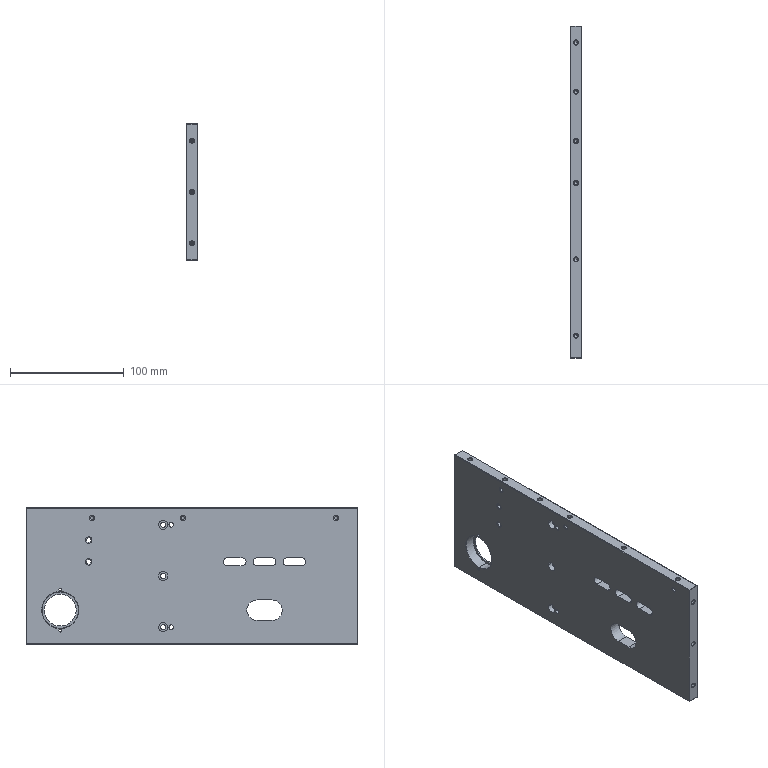Part | NX | 1 solid | 200 faces | box 10 x 291.5 x 120 mm | volume 329656 mm3 | cone 88 | cylinder 83 | plane 29 | commonest cylinder face diameters 3.3 x43 7 x9 4.5 x6 8 x6 2.5 x4 4 x4